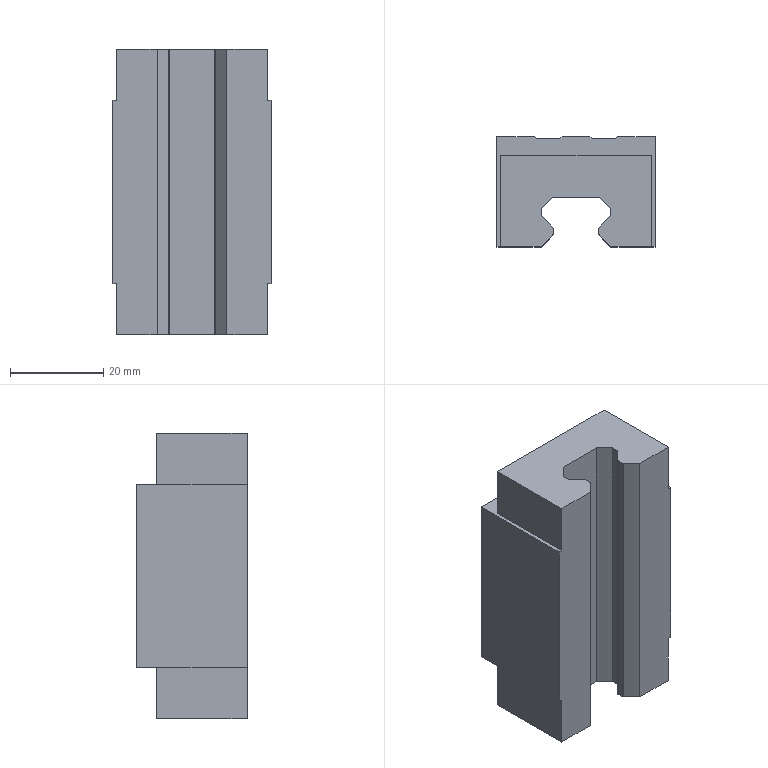Part | STEP file | Slider HGH15CA ( HGH15CA) | 1 solid | 50 faces | box 34 x 23.7 x 61.4 mm | volume 37112 mm3 | plane 38 | cylinder 12 | commonest cylinder face diameters 3.2 x8 0.8 x4
STEP:
#1=CARTESIAN_POINT('',(-26.228,-14.514,42.1));
#2=VERTEX_POINT('',#1);
#3=CARTESIAN_POINT('',(-26.228,-14.514,45.3));
#4=VERTEX_POINT('',#3);
#5=CARTESIAN_POINT('',(-26.228,-14.514,43.7));
#6=DIRECTION('',(0.,1.,0.));
#7=DIRECTION('',(0.,0.,1.));
#8=AXIS2_PLACEMENT_3D('',#5,#6,#7);
#9=CIRCLE('',#8,1.6);
#10=EDGE_CURVE('',#2,#4,#9,.T.);
#11=ORIENTED_EDGE('',*,*,#10,.F.);
#12=CARTESIAN_POINT('',(-26.228,-9.514,42.1));
#13=VERTEX_POINT('',#12);
#14=CARTESIAN_POINT('',(-26.228,-14.514,42.1));
#15=DIRECTION('',(0.,1.,0.));
#16=VECTOR('',#15,1000.);
#17=LINE('',#14,#16);
#18=EDGE_CURVE('',#2,#13,#17,.T.);
#19=ORIENTED_EDGE('',*,*,#18,.T.);
#20=CARTESIAN_POINT('',(-26.228,-9.514,45.3));
#21=VERTEX_POINT('',#20);
#22=CARTESIAN_POINT('',(-26.228,-9.514,43.7));
#23=DIRECTION('',(0.,1.,0.));
#24=DIRECTION('',(0.,0.,1.));
#25=AXIS2_PLACEMENT_3D('',#22,#23,#24);
#26=CIRCLE('',#25,1.6);
#27=EDGE_CURVE('',#13,#21,#26,.T.);
#28=ORIENTED_EDGE('',*,*,#27,.T.);
#29=CARTESIAN_POINT('',(-26.228,-14.514,45.3));
#30=DIRECTION('',(0.,1.,0.));
#31=VECTOR('',#30,1000.);
#32=LINE('',#29,#31);
#33=EDGE_CURVE('',#4,#21,#32,.T.);
#34=ORIENTED_EDGE('',*,*,#33,.F.);
#35=EDGE_LOOP('',(#11,#19,#28,#34));
#36=FACE_OUTER_BOUND('',#35,.T.);
#37=CARTESIAN_POINT('',(-26.228,-14.514,43.7));
#38=DIRECTION('',(0.,1.,0.));
#39=DIRECTION('',(0.,0.,1.));
#40=AXIS2_PLACEMENT_3D('',#37,#38,#39);
#41=CYLINDRICAL_SURFACE('',#40,1.6);
#42=ADVANCED_FACE('',(#36),#41,.F.);
#43=CARTESIAN_POINT('',(-26.228,-14.514,16.1));
#44=VERTEX_POINT('',#43);
#45=CARTESIAN_POINT('',(-26.228,-14.514,19.3));
#46=VERTEX_POINT('',#45);
#47=CARTESIAN_POINT('',(-26.228,-14.514,17.7));
#48=DIRECTION('',(0.,1.,0.));
#49=DIRECTION('',(0.,0.,1.));
#50=AXIS2_PLACEMENT_3D('',#47,#48,#49);
#51=CIRCLE('',#50,1.6);
#52=EDGE_CURVE('',#44,#46,#51,.T.);
#53=ORIENTED_EDGE('',*,*,#52,.F.);
#54=CARTESIAN_POINT('',(-26.228,-9.514,16.1));
#55=VERTEX_POINT('',#54);
#56=CARTESIAN_POINT('',(-26.228,-14.514,16.1));
#57=DIRECTION('',(0.,1.,0.));
#58=VECTOR('',#57,1000.);
#59=LINE('',#56,#58);
#60=EDGE_CURVE('',#44,#55,#59,.T.);
#61=ORIENTED_EDGE('',*,*,#60,.T.);
#62=CARTESIAN_POINT('',(-26.228,-9.514,19.3));
#63=VERTEX_POINT('',#62);
#64=CARTESIAN_POINT('',(-26.228,-9.514,17.7));
#65=DIRECTION('',(0.,1.,0.));
#66=DIRECTION('',(0.,0.,1.));
#67=AXIS2_PLACEMENT_3D('',#64,#65,#66);
#68=CIRCLE('',#67,1.6);
#69=EDGE_CURVE('',#55,#63,#68,.T.);
#70=ORIENTED_EDGE('',*,*,#69,.T.);
#71=CARTESIAN_POINT('',(-26.228,-14.514,19.3));
#72=DIRECTION('',(0.,1.,0.));
#73=VECTOR('',#72,1000.);
#74=LINE('',#71,#73);
#75=EDGE_CURVE('',#46,#63,#74,.T.);
#76=ORIENTED_EDGE('',*,*,#75,.F.);
#77=EDGE_LOOP('',(#53,#61,#70,#76));
#78=FACE_OUTER_BOUND('',#77,.T.);
#79=CARTESIAN_POINT('',(-26.228,-14.514,17.7));
#80=DIRECTION('',(0.,1.,0.));
#81=DIRECTION('',(0.,0.,1.));
#82=AXIS2_PLACEMENT_3D('',#79,#80,#81);
#83=CYLINDRICAL_SURFACE('',#82,1.6);
#84=ADVANCED_FACE('',(#78),#83,.F.);
#85=CARTESIAN_POINT('',(-0.2285,-14.514,42.1));
#86=VERTEX_POINT('',#85);
#87=CARTESIAN_POINT('',(-0.2285,-14.514,45.3));
#88=VERTEX_POINT('',#87);
#89=CARTESIAN_POINT('',(-0.2285,-14.514,43.7));
#90=DIRECTION('',(0.,1.,0.));
#91=DIRECTION('',(0.,0.,1.));
#92=AXIS2_PLACEMENT_3D('',#89,#90,#91);
#93=CIRCLE('',#92,1.6);
#94=EDGE_CURVE('',#86,#88,#93,.T.);
#95=ORIENTED_EDGE('',*,*,#94,.F.);
#96=CARTESIAN_POINT('',(-0.2285,-9.514,42.1));
#97=VERTEX_POINT('',#96);
#98=CARTESIAN_POINT('',(-0.2285,-14.514,42.1));
#99=DIRECTION('',(0.,1.,0.));
#100=VECTOR('',#99,1000.);
#101=LINE('',#98,#100);
#102=EDGE_CURVE('',#86,#97,#101,.T.);
#103=ORIENTED_EDGE('',*,*,#102,.T.);
#104=CARTESIAN_POINT('',(-0.2285,-9.514,45.3));
#105=VERTEX_POINT('',#104);
#106=CARTESIAN_POINT('',(-0.2285,-9.514,43.7));
#107=DIRECTION('',(0.,1.,0.));
#108=DIRECTION('',(0.,0.,1.));
#109=AXIS2_PLACEMENT_3D('',#106,#107,#108);
#110=CIRCLE('',#109,1.6);
#111=EDGE_CURVE('',#97,#105,#110,.T.);
#112=ORIENTED_EDGE('',*,*,#111,.T.);
#113=CARTESIAN_POINT('',(-0.2285,-14.514,45.3));
#114=DIRECTION('',(0.,1.,0.));
#115=VECTOR('',#114,1000.);
#116=LINE('',#113,#115);
#117=EDGE_CURVE('',#88,#105,#116,.T.);
#118=ORIENTED_EDGE('',*,*,#117,.F.);
#119=EDGE_LOOP('',(#95,#103,#112,#118));
#120=FACE_OUTER_BOUND('',#119,.T.);
#121=CARTESIAN_POINT('',(-0.2285,-14.514,43.7));
#122=DIRECTION('',(0.,1.,0.));
#123=DIRECTION('',(0.,0.,1.));
#124=AXIS2_PLACEMENT_3D('',#121,#122,#123);
#125=CYLINDRICAL_SURFACE('',#124,1.6);
#126=ADVANCED_FACE('',(#120),#125,.F.);
#127=CARTESIAN_POINT('',(-0.2285,-14.514,16.1));
#128=VERTEX_POINT('',#127);
#129=CARTESIAN_POINT('',(-0.2285,-14.514,19.3));
#130=VERTEX_POINT('',#129);
#131=CARTESIAN_POINT('',(-0.2285,-14.514,17.7));
#132=DIRECTION('',(0.,1.,0.));
#133=DIRECTION('',(0.,0.,1.));
#134=AXIS2_PLACEMENT_3D('',#131,#132,#133);
#135=CIRCLE('',#134,1.6);
#136=EDGE_CURVE('',#128,#130,#135,.T.);
#137=ORIENTED_EDGE('',*,*,#136,.F.);
#138=CARTESIAN_POINT('',(-0.2285,-9.514,16.1));
#139=VERTEX_POINT('',#138);
#140=CARTESIAN_POINT('',(-0.2285,-14.514,16.1));
#141=DIRECTION('',(0.,1.,0.));
#142=VECTOR('',#141,1000.);
#143=LINE('',#140,#142);
#144=EDGE_CURVE('',#128,#139,#143,.T.);
#145=ORIENTED_EDGE('',*,*,#144,.T.);
#146=CARTESIAN_POINT('',(-0.2285,-9.514,19.3));
#147=VERTEX_POINT('',#146);
#148=CARTESIAN_POINT('',(-0.2285,-9.514,17.7));
#149=DIRECTION('',(0.,1.,0.));
#150=DIRECTION('',(0.,0.,1.));
#151=AXIS2_PLACEMENT_3D('',#148,#149,#150);
#152=CIRCLE('',#151,1.6);
#153=EDGE_CURVE('',#139,#147,#152,.T.);
#154=ORIENTED_EDGE('',*,*,#153,.T.);
#155=CARTESIAN_POINT('',(-0.2285,-14.514,19.3));
#156=DIRECTION('',(0.,1.,0.));
#157=VECTOR('',#156,1000.);
#158=LINE('',#155,#157);
#159=EDGE_CURVE('',#130,#147,#158,.T.);
#160=ORIENTED_EDGE('',*,*,#159,.F.);
#161=EDGE_LOOP('',(#137,#145,#154,#160));
#162=FACE_OUTER_BOUND('',#161,.T.);
#163=CARTESIAN_POINT('',(-0.2285,-14.514,17.7));
#164=DIRECTION('',(0.,1.,0.));
#165=DIRECTION('',(0.,0.,1.));
#166=AXIS2_PLACEMENT_3D('',#163,#164,#165);
#167=CYLINDRICAL_SURFACE('',#166,1.6);
#168=ADVANCED_FACE('',(#162),#167,.F.);
#169=CARTESIAN_POINT('',(-29.428,-33.214,0.));
#170=VERTEX_POINT('',#169);
#171=CARTESIAN_POINT('',(-20.728,-33.214,0.));
#172=VERTEX_POINT('',#171);
#173=CARTESIAN_POINT('',(-29.428,-33.214,0.));
#174=DIRECTION('',(1.,0.,0.));
#175=VECTOR('',#174,1000.);
#176=LINE('',#173,#175);
#177=EDGE_CURVE('',#170,#172,#176,.T.);
#178=ORIENTED_EDGE('',*,*,#177,.T.);
#179=CARTESIAN_POINT('',(-20.728,-33.214,61.4));
#180=VERTEX_POINT('',#179);
#181=CARTESIAN_POINT('',(-20.728,-33.214,61.4));
#182=DIRECTION('',(0.,0.,-1.));
#183=VECTOR('',#182,1000.);
#184=LINE('',#181,#183);
#185=EDGE_CURVE('',#180,#172,#184,.T.);
#186=ORIENTED_EDGE('',*,*,#185,.F.);
#187=CARTESIAN_POINT('',(-29.428,-33.214,61.4));
#188=VERTEX_POINT('',#187);
#189=CARTESIAN_POINT('',(-29.428,-33.214,61.4));
#190=DIRECTION('',(1.,0.,0.));
#191=VECTOR('',#190,1000.);
#192=LINE('',#189,#191);
#193=EDGE_CURVE('',#188,#180,#192,.T.);
#194=ORIENTED_EDGE('',*,*,#193,.F.);
#195=CARTESIAN_POINT('',(-29.428,-33.214,50.4));
#196=VERTEX_POINT('',#195);
#197=CARTESIAN_POINT('',(-29.428,-33.214,50.4));
#198=DIRECTION('',(0.,0.,1.));
#199=VECTOR('',#198,1000.);
#200=LINE('',#197,#199);
#201=EDGE_CURVE('',#196,#188,#200,.T.);
#202=ORIENTED_EDGE('',*,*,#201,.F.);
#203=CARTESIAN_POINT('',(-30.228,-33.214,50.4));
#204=VERTEX_POINT('',#203);
#205=CARTESIAN_POINT('',(-30.228,-33.214,50.4));
#206=DIRECTION('',(1.,0.,0.));
#207=VECTOR('',#206,1000.);
#208=LINE('',#205,#207);
#209=EDGE_CURVE('',#204,#196,#208,.T.);
#210=ORIENTED_EDGE('',*,*,#209,.F.);
#211=CARTESIAN_POINT('',(-30.228,-33.214,11.));
#212=VERTEX_POINT('',#211);
#213=CARTESIAN_POINT('',(-30.228,-33.214,50.4));
#214=DIRECTION('',(0.,0.,-1.));
#215=VECTOR('',#214,1000.);
#216=LINE('',#213,#215);
#217=EDGE_CURVE('',#204,#212,#216,.T.);
#218=ORIENTED_EDGE('',*,*,#217,.T.);
#219=CARTESIAN_POINT('',(-29.428,-33.214,11.));
#220=VERTEX_POINT('',#219);
#221=CARTESIAN_POINT('',(-30.228,-33.214,11.));
#222=DIRECTION('',(1.,0.,0.));
#223=VECTOR('',#222,1000.);
#224=LINE('',#221,#223);
#225=EDGE_CURVE('',#212,#220,#224,.T.);
#226=ORIENTED_EDGE('',*,*,#225,.T.);
#227=CARTESIAN_POINT('',(-29.428,-33.214,11.));
#228=DIRECTION('',(0.,0.,-1.));
#229=VECTOR('',#228,1000.);
#230=LINE('',#227,#229);
#231=EDGE_CURVE('',#220,#170,#230,.T.);
#232=ORIENTED_EDGE('',*,*,#231,.T.);
#233=EDGE_LOOP('',(#178,#186,#194,#202,#210,#218,#226,#232));
#234=FACE_OUTER_BOUND('',#233,.T.);
#235=CARTESIAN_POINT('',(-29.428,-33.214,11.));
#236=DIRECTION('',(0.,1.,0.));
#237=DIRECTION('',(0.,0.,1.));
#238=AXIS2_PLACEMENT_3D('',#235,#236,#237);
#239=PLANE('',#238);
#240=ADVANCED_FACE('',(#234),#239,.F.);
#241=CARTESIAN_POINT('',(-21.728,-10.014,11.));
#242=VERTEX_POINT('',#241);
#243=CARTESIAN_POINT('',(-22.228,-9.514,11.));
#244=VERTEX_POINT('',#243);
#245=CARTESIAN_POINT('',(-14.378,-17.364,11.));
#246=DIRECTION('',(-0.7071,0.7071,0.));
#247=VECTOR('',#246,1000.);
#248=LINE('',#245,#247);
#249=EDGE_CURVE('',#242,#244,#248,.T.);
#250=ORIENTED_EDGE('',*,*,#249,.F.);
#251=CARTESIAN_POINT('',(-16.728,-10.014,11.));
#252=VERTEX_POINT('',#251);
#253=CARTESIAN_POINT('',(-30.228,-10.014,11.));
#254=DIRECTION('',(-1.,0.,0.));
#255=VECTOR('',#254,1000.);
#256=LINE('',#253,#255);
#257=EDGE_CURVE('',#252,#242,#256,.T.);
#258=ORIENTED_EDGE('',*,*,#257,.F.);
#259=CARTESIAN_POINT('',(-16.228,-9.514,11.));
#260=VERTEX_POINT('',#259);
#261=CARTESIAN_POINT('',(-35.078,-28.364,11.));
#262=DIRECTION('',(-0.7071,-0.7071,0.));
#263=VECTOR('',#262,1000.);
#264=LINE('',#261,#263);
#265=EDGE_CURVE('',#260,#252,#264,.T.);
#266=ORIENTED_EDGE('',*,*,#265,.F.);
#267=CARTESIAN_POINT('',(-10.228,-9.514,11.));
#268=VERTEX_POINT('',#267);
#269=CARTESIAN_POINT('',(-30.228,-9.514,11.));
#270=DIRECTION('',(-1.,0.,0.));
#271=VECTOR('',#270,1000.);
#272=LINE('',#269,#271);
#273=EDGE_CURVE('',#268,#260,#272,.T.);
#274=ORIENTED_EDGE('',*,*,#273,.F.);
#275=CARTESIAN_POINT('',(-9.728,-10.014,11.));
#276=VERTEX_POINT('',#275);
#277=CARTESIAN_POINT('',(-8.378,-11.364,11.));
#278=DIRECTION('',(0.7071,-0.7071,0.));
#279=VECTOR('',#278,1000.);
#280=LINE('',#277,#279);
#281=EDGE_CURVE('',#268,#276,#280,.T.);
#282=ORIENTED_EDGE('',*,*,#281,.T.);
#283=CARTESIAN_POINT('',(-4.728,-10.014,11.));
#284=VERTEX_POINT('',#283);
#285=CARTESIAN_POINT('',(-30.228,-10.014,11.));
#286=DIRECTION('',(1.,0.,0.));
#287=VECTOR('',#286,1000.);
#288=LINE('',#285,#287);
#289=EDGE_CURVE('',#276,#284,#288,.T.);
#290=ORIENTED_EDGE('',*,*,#289,.T.);
#291=CARTESIAN_POINT('',(-4.228,-9.514,11.));
#292=VERTEX_POINT('',#291);
#293=CARTESIAN_POINT('',(-29.078,-34.364,11.));
#294=DIRECTION('',(0.7071,0.7071,0.));
#295=VECTOR('',#294,1000.);
#296=LINE('',#293,#295);
#297=EDGE_CURVE('',#284,#292,#296,.T.);
#298=ORIENTED_EDGE('',*,*,#297,.T.);
#299=CARTESIAN_POINT('',(3.772,-9.514,11.));
#300=VERTEX_POINT('',#299);
#301=CARTESIAN_POINT('',(-30.228,-9.514,11.));
#302=DIRECTION('',(-1.,0.,0.));
#303=VECTOR('',#302,1000.);
#304=LINE('',#301,#303);
#305=EDGE_CURVE('',#300,#292,#304,.T.);
#306=ORIENTED_EDGE('',*,*,#305,.F.);
#307=CARTESIAN_POINT('',(3.772,-33.214,11.));
#308=VERTEX_POINT('',#307);
#309=CARTESIAN_POINT('',(3.772,-9.514,11.));
#310=DIRECTION('',(0.,1.,0.));
#311=VECTOR('',#310,1000.);
#312=LINE('',#309,#311);
#313=EDGE_CURVE('',#308,#300,#312,.T.);
#314=ORIENTED_EDGE('',*,*,#313,.F.);
#315=CARTESIAN_POINT('',(2.972,-33.214,11.));
#316=VERTEX_POINT('',#315);
#317=CARTESIAN_POINT('',(-30.228,-33.214,11.));
#318=DIRECTION('',(1.,0.,0.));
#319=VECTOR('',#318,1000.);
#320=LINE('',#317,#319);
#321=EDGE_CURVE('',#316,#308,#320,.T.);
#322=ORIENTED_EDGE('',*,*,#321,.F.);
#323=CARTESIAN_POINT('',(2.972,-13.684,11.));
#324=VERTEX_POINT('',#323);
#325=CARTESIAN_POINT('',(2.972,-13.684,11.));
#326=DIRECTION('',(0.,1.,0.));
#327=VECTOR('',#326,1000.);
#328=LINE('',#325,#327);
#329=EDGE_CURVE('',#316,#324,#328,.T.);
#330=ORIENTED_EDGE('',*,*,#329,.T.);
#331=CARTESIAN_POINT('',(-29.428,-13.684,11.));
#332=VERTEX_POINT('',#331);
#333=CARTESIAN_POINT('',(-29.428,-13.684,11.));
#334=DIRECTION('',(-1.,0.,0.));
#335=VECTOR('',#334,1000.);
#336=LINE('',#333,#335);
#337=EDGE_CURVE('',#324,#332,#336,.T.);
#338=ORIENTED_EDGE('',*,*,#337,.T.);
#339=CARTESIAN_POINT('',(-29.428,-13.684,11.));
#340=DIRECTION('',(0.,-1.,0.));
#341=VECTOR('',#340,1000.);
#342=LINE('',#339,#341);
#343=EDGE_CURVE('',#332,#220,#342,.T.);
#344=ORIENTED_EDGE('',*,*,#343,.T.);
#345=ORIENTED_EDGE('',*,*,#225,.F.);
#346=CARTESIAN_POINT('',(-30.228,-9.514,11.));
#347=VERTEX_POINT('',#346);
#348=CARTESIAN_POINT('',(-30.228,-9.514,11.));
#349=DIRECTION('',(0.,-1.,0.));
#350=VECTOR('',#349,1000.);
#351=LINE('',#348,#350);
#352=EDGE_CURVE('',#347,#212,#351,.T.);
#353=ORIENTED_EDGE('',*,*,#352,.F.);
#354=CARTESIAN_POINT('',(-30.228,-9.514,11.));
#355=DIRECTION('',(-1.,0.,0.));
#356=VECTOR('',#355,1000.);
#357=LINE('',#354,#356);
#358=EDGE_CURVE('',#244,#347,#357,.T.);
#359=ORIENTED_EDGE('',*,*,#358,.F.);
#360=EDGE_LOOP('',(#250,#258,#266,#274,#282,#290,#298,#306,#314,#322,#330,#338,#344,#345,#353,#359));
#361=FACE_OUTER_BOUND('',#360,.T.);
#362=CARTESIAN_POINT('',(-30.228,-33.214,11.));
#363=DIRECTION('',(0.,0.,1.));
#364=DIRECTION('',(1.,0.,0.));
#365=AXIS2_PLACEMENT_3D('',#362,#363,#364);
#366=PLANE('',#365);
#367=ADVANCED_FACE('',(#361),#366,.F.);
#368=CARTESIAN_POINT('',(-26.228,-9.514,43.7));
#369=DIRECTION('',(0.,1.,0.));
#370=DIRECTION('',(0.,0.,1.));
#371=AXIS2_PLACEMENT_3D('',#368,#369,#370);
#372=CIRCLE('',#371,1.6);
#373=EDGE_CURVE('',#21,#13,#372,.T.);
#374=ORIENTED_EDGE('',*,*,#373,.F.);
#375=ORIENTED_EDGE('',*,*,#27,.F.);
#376=EDGE_LOOP('',(#374,#375));
#377=FACE_BOUND('',#376,.T.);
#378=CARTESIAN_POINT('',(-26.228,-9.514,17.7));
#379=DIRECTION('',(0.,1.,0.));
#380=DIRECTION('',(0.,0.,1.));
#381=AXIS2_PLACEMENT_3D('',#378,#379,#380);
#382=CIRCLE('',#381,1.6);
#383=EDGE_CURVE('',#63,#55,#382,.T.);
#384=ORIENTED_EDGE('',*,*,#383,.F.);
#385=ORIENTED_EDGE('',*,*,#69,.F.);
#386=EDGE_LOOP('',(#384,#385));
#387=FACE_BOUND('',#386,.T.);
#388=CARTESIAN_POINT('',(-22.228,-9.514,50.4));
#389=VERTEX_POINT('',#388);
#390=CARTESIAN_POINT('',(-22.228,-9.514,-0.000025));
#391=DIRECTION('',(0.,0.,1.));
#392=VECTOR('',#391,1000.);
#393=LINE('',#390,#392);
#394=EDGE_CURVE('',#244,#389,#393,.T.);
#395=ORIENTED_EDGE('',*,*,#394,.F.);
#396=ORIENTED_EDGE('',*,*,#358,.T.);
#397=CARTESIAN_POINT('',(-30.228,-9.514,50.4));
#398=VERTEX_POINT('',#397);
#399=CARTESIAN_POINT('',(-30.228,-9.514,50.4));
#400=DIRECTION('',(0.,0.,-1.));
#401=VECTOR('',#400,1000.);
#402=LINE('',#399,#401);
#403=EDGE_CURVE('',#398,#347,#402,.T.);
#404=ORIENTED_EDGE('',*,*,#403,.F.);
#405=CARTESIAN_POINT('',(-30.228,-9.514,50.4));
#406=DIRECTION('',(-1.,0.,0.));
#407=VECTOR('',#406,1000.);
#408=LINE('',#405,#407);
#409=EDGE_CURVE('',#389,#398,#408,.T.);
#410=ORIENTED_EDGE('',*,*,#409,.F.);
#411=EDGE_LOOP('',(#395,#396,#404,#410));
#412=FACE_OUTER_BOUND('',#411,.T.);
#413=CARTESIAN_POINT('',(-30.228,-9.514,50.4));
#414=DIRECTION('',(0.,-1.,0.));
#415=DIRECTION('',(0.,0.,-1.));
#416=AXIS2_PLACEMENT_3D('',#413,#414,#415);
#417=PLANE('',#416);
#418=ADVANCED_FACE('',(#377,#387,#412),#417,.F.);
#419=CARTESIAN_POINT('',(-16.228,-9.514,50.4));
#420=VERTEX_POINT('',#419);
#421=CARTESIAN_POINT('',(-16.228,-9.514,-0.000025));
#422=DIRECTION('',(0.,0.,1.));
#423=VECTOR('',#422,1000.);
#424=LINE('',#421,#423);
#425=EDGE_CURVE('',#260,#420,#424,.T.);
#426=ORIENTED_EDGE('',*,*,#425,.T.);
#427=CARTESIAN_POINT('',(-10.228,-9.514,50.4));
#428=VERTEX_POINT('',#427);
#429=CARTESIAN_POINT('',(-30.228,-9.514,50.4));
#430=DIRECTION('',(-1.,0.,0.));
#431=VECTOR('',#430,1000.);
#432=LINE('',#429,#431);
#433=EDGE_CURVE('',#428,#420,#432,.T.);
#434=ORIENTED_EDGE('',*,*,#433,.F.);
#435=CARTESIAN_POINT('',(-10.228,-9.514,-0.000025));
#436=DIRECTION('',(0.,0.,1.));
#437=VECTOR('',#436,1000.);
#438=LINE('',#435,#437);
#439=EDGE_CURVE('',#268,#428,#438,.T.);
#440=ORIENTED_EDGE('',*,*,#439,.F.);
#441=ORIENTED_EDGE('',*,*,#273,.T.);
#442=EDGE_LOOP('',(#426,#434,#440,#441));
#443=FACE_OUTER_BOUND('',#442,.T.);
#444=CARTESIAN_POINT('',(-30.228,-9.514,50.4));
#445=DIRECTION('',(0.,-1.,0.));
#446=DIRECTION('',(0.,0.,-1.));
#447=AXIS2_PLACEMENT_3D('',#444,#445,#446);
#448=PLANE('',#447);
#449=ADVANCED_FACE('',(#443),#448,.F.);
#450=CARTESIAN_POINT('',(-16.728,-10.014,50.4));
#451=VERTEX_POINT('',#450);
#452=CARTESIAN_POINT('',(-21.728,-10.014,50.4));
#453=VERTEX_POINT('',#452);
#454=CARTESIAN_POINT('',(-16.728,-10.014,50.4));
#455=DIRECTION('',(-1.,0.,0.));
#456=VECTOR('',#455,1000.);
#457=LINE('',#454,#456);
#458=EDGE_CURVE('',#451,#453,#457,.T.);
#459=ORIENTED_EDGE('',*,*,#458,.T.);
#460=CARTESIAN_POINT('',(-21.728,-10.014,50.4));
#461=DIRECTION('',(-0.7071,0.7071,0.));
#462=VECTOR('',#461,1000.);
#463=LINE('',#460,#462);
#464=EDGE_CURVE('',#453,#389,#463,.T.);
#465=ORIENTED_EDGE('',*,*,#464,.T.);
#466=ORIENTED_EDGE('',*,*,#409,.T.);
#467=CARTESIAN_POINT('',(-30.228,-9.514,50.4));
#468=DIRECTION('',(0.,-1.,0.));
#469=VECTOR('',#468,1000.);
#470=LINE('',#467,#469);
#471=EDGE_CURVE('',#398,#204,#470,.T.);
#472=ORIENTED_EDGE('',*,*,#471,.T.);
#473=ORIENTED_EDGE('',*,*,#209,.T.);
#474=CARTESIAN_POINT('',(-29.428,-13.684,50.4));
#475=VERTEX_POINT('',#474);
#476=CARTESIAN_POINT('',(-29.428,-13.684,50.4));
#477=DIRECTION('',(0.,-1.,0.));
#478=VECTOR('',#477,1000.);
#479=LINE('',#476,#478);
#480=EDGE_CURVE('',#475,#196,#479,.T.);
#481=ORIENTED_EDGE('',*,*,#480,.F.);
#482=CARTESIAN_POINT('',(2.972,-13.684,50.4));
#483=VERTEX_POINT('',#482);
#484=CARTESIAN_POINT('',(-29.428,-13.684,50.4));
#485=DIRECTION('',(-1.,0.,0.));
#486=VECTOR('',#485,1000.);
#487=LINE('',#484,#486);
#488=EDGE_CURVE('',#483,#475,#487,.T.);
#489=ORIENTED_EDGE('',*,*,#488,.F.);
#490=CARTESIAN_POINT('',(2.972,-33.214,50.4));
#491=VERTEX_POINT('',#490);
#492=CARTESIAN_POINT('',(2.972,-13.684,50.4));
#493=DIRECTION('',(0.,1.,0.));
#494=VECTOR('',#493,1000.);
#495=LINE('',#492,#494);
#496=EDGE_CURVE('',#491,#483,#495,.T.);
#497=ORIENTED_EDGE('',*,*,#496,.F.);
#498=CARTESIAN_POINT('',(3.772,-33.214,50.4));
#499=VERTEX_POINT('',#498);
#500=CARTESIAN_POINT('',(-30.228,-33.214,50.4));
#501=DIRECTION('',(1.,0.,0.));
#502=VECTOR('',#501,1000.);
#503=LINE('',#500,#502);
#504=EDGE_CURVE('',#491,#499,#503,.T.);
#505=ORIENTED_EDGE('',*,*,#504,.T.);
#506=CARTESIAN_POINT('',(3.772,-9.514,50.4));
#507=VERTEX_POINT('',#506);
#508=CARTESIAN_POINT('',(3.772,-9.514,50.4));
#509=DIRECTION('',(0.,1.,0.));
#510=VECTOR('',#509,1000.);
#511=LINE('',#508,#510);
#512=EDGE_CURVE('',#499,#507,#511,.T.);
#513=ORIENTED_EDGE('',*,*,#512,.T.);
#514=CARTESIAN_POINT('',(-4.228,-9.514,50.4));
#515=VERTEX_POINT('',#514);
#516=CARTESIAN_POINT('',(-30.228,-9.514,50.4));
#517=DIRECTION('',(-1.,0.,0.));
#518=VECTOR('',#517,1000.);
#519=LINE('',#516,#518);
#520=EDGE_CURVE('',#507,#515,#519,.T.);
#521=ORIENTED_EDGE('',*,*,#520,.T.);
#522=CARTESIAN_POINT('',(-4.728,-10.014,50.4));
#523=VERTEX_POINT('',#522);
#524=CARTESIAN_POINT('',(-4.728,-10.014,50.4));
#525=DIRECTION('',(0.7071,0.7071,0.));
#526=VECTOR('',#525,1000.);
#527=LINE('',#524,#526);
#528=EDGE_CURVE('',#523,#515,#527,.T.);
#529=ORIENTED_EDGE('',*,*,#528,.F.);
#530=CARTESIAN_POINT('',(-9.728,-10.014,50.4));
#531=VERTEX_POINT('',#530);
#532=CARTESIAN_POINT('',(-9.728,-10.014,50.4));
#533=DIRECTION('',(1.,0.,0.));
#534=VECTOR('',#533,1000.);
#535=LINE('',#532,#534);
#536=EDGE_CURVE('',#531,#523,#535,.T.);
#537=ORIENTED_EDGE('',*,*,#536,.F.);
#538=CARTESIAN_POINT('',(-9.728,-10.014,50.4));
#539=DIRECTION('',(0.7071,-0.7071,0.));
#540=VECTOR('',#539,1000.);
#541=LINE('',#538,#540);
#542=EDGE_CURVE('',#428,#531,#541,.T.);
#543=ORIENTED_EDGE('',*,*,#542,.F.);
#544=ORIENTED_EDGE('',*,*,#433,.T.);
#545=CARTESIAN_POINT('',(-16.728,-10.014,50.4));
#546=DIRECTION('',(-0.7071,-0.7071,0.));
#547=VECTOR('',#546,1000.);
#548=LINE('',#545,#547);
#549=EDGE_CURVE('',#420,#451,#548,.T.);
#550=ORIENTED_EDGE('',*,*,#549,.T.);
#551=EDGE_LOOP('',(#459,#465,#466,#472,#473,#481,#489,#497,#505,#513,#521,#529,#537,#543,#544,#550));
#552=FACE_OUTER_BOUND('',#551,.T.);
#553=CARTESIAN_POINT('',(-30.228,-33.214,50.4));
#554=DIRECTION('',(0.,0.,1.));
#555=DIRECTION('',(1.,0.,0.));
#556=AXIS2_PLACEMENT_3D('',#553,#554,#555);
#557=PLANE('',#556);
#558=ADVANCED_FACE('',(#552),#557,.T.);
#559=CARTESIAN_POINT('',(-0.2285,-9.514,43.7));
#560=DIRECTION('',(0.,1.,0.));
#561=DIRECTION('',(0.,0.,1.));
#562=AXIS2_PLACEMENT_3D('',#559,#560,#561);
#563=CIRCLE('',#562,1.6);
#564=EDGE_CURVE('',#105,#97,#563,.T.);
#565=ORIENTED_EDGE('',*,*,#564,.F.);
#566=ORIENTED_EDGE('',*,*,#111,.F.);
#567=EDGE_LOOP('',(#565,#566));
#568=FACE_BOUND('',#567,.T.);
#569=CARTESIAN_POINT('',(-0.2285,-9.514,17.7));
#570=DIRECTION('',(0.,1.,0.));
#571=DIRECTION('',(0.,0.,1.));
#572=AXIS2_PLACEMENT_3D('',#569,#570,#571);
#573=CIRCLE('',#572,1.6);
#574=EDGE_CURVE('',#147,#139,#573,.T.);
#575=ORIENTED_EDGE('',*,*,#574,.F.);
#576=ORIENTED_EDGE('',*,*,#153,.F.);
#577=EDGE_LOOP('',(#575,#576));
#578=FACE_BOUND('',#577,.T.);
#579=ORIENTED_EDGE('',*,*,#305,.T.);
#580=CARTESIAN_POINT('',(-4.228,-9.514,-0.000025));
#581=DIRECTION('',(0.,0.,1.));
#582=VECTOR('',#581,1000.);
#583=LINE('',#580,#582);
#584=EDGE_CURVE('',#292,#515,#583,.T.);
#585=ORIENTED_EDGE('',*,*,#584,.T.);
#586=ORIENTED_EDGE('',*,*,#520,.F.);
#587=CARTESIAN_POINT('',(3.772,-9.514,50.4));
#588=DIRECTION('',(0.,0.,-1.));
#589=VECTOR('',#588,1000.);
#590=LINE('',#587,#589);
#591=EDGE_CURVE('',#507,#300,#590,.T.);
#592=ORIENTED_EDGE('',*,*,#591,.T.);
#593=EDGE_LOOP('',(#579,#585,#586,#592));
#594=FACE_OUTER_BOUND('',#593,.T.);
#595=CARTESIAN_POINT('',(-30.228,-9.514,50.4));
#596=DIRECTION('',(0.,-1.,0.));
#597=DIRECTION('',(0.,0.,-1.));
#598=AXIS2_PLACEMENT_3D('',#595,#596,#597);
#599=PLANE('',#598);
#600=ADVANCED_FACE('',(#568,#578,#594),#599,.F.);
#601=CARTESIAN_POINT('',(-29.428,-13.684,0.));
#602=VERTEX_POINT('',#601);
#603=CARTESIAN_POINT('',(-29.428,-13.684,0.));
#604=DIRECTION('',(0.,-1.,0.));
#605=VECTOR('',#604,1000.);
#606=LINE('',#603,#605);
#607=EDGE_CURVE('',#602,#170,#606,.T.);
#608=ORIENTED_EDGE('',*,*,#607,.T.);
#609=ORIENTED_EDGE('',*,*,#231,.F.);
#610=ORIENTED_EDGE('',*,*,#343,.F.);
#611=CARTESIAN_POINT('',(-29.428,-13.684,11.));
#612=DIRECTION('',(0.,0.,-1.));
#613=VECTOR('',#612,1000.);
#614=LINE('',#611,#613);
#615=EDGE_CURVE('',#332,#602,#614,.T.);
#616=ORIENTED_EDGE('',*,*,#615,.T.);
#617=EDGE_LOOP('',(#608,#609,#610,#616));
#618=FACE_OUTER_BOUND('',#617,.T.);
#619=CARTESIAN_POINT('',(-29.428,-13.684,11.));
#620=DIRECTION('',(1.,0.,0.));
#621=DIRECTION('',(0.,1.,0.));
#622=AXIS2_PLACEMENT_3D('',#619,#620,#621);
#623=PLANE('',#622);
#624=ADVANCED_FACE('',(#618),#623,.F.);
#625=CARTESIAN_POINT('',(-5.728,-33.214,61.4));
#626=VERTEX_POINT('',#625);
#627=CARTESIAN_POINT('',(2.972,-33.214,61.4));
#628=VERTEX_POINT('',#627);
#629=CARTESIAN_POINT('',(-29.428,-33.214,61.4));
#630=DIRECTION('',(1.,0.,0.));
#631=VECTOR('',#630,1000.);
#632=LINE('',#629,#631);
#633=EDGE_CURVE('',#626,#628,#632,.T.);
#634=ORIENTED_EDGE('',*,*,#633,.F.);
#635=CARTESIAN_POINT('',(-5.728,-33.214,0.));
#636=VERTEX_POINT('',#635);
#637=CARTESIAN_POINT('',(-5.728,-33.214,61.4));
#638=DIRECTION('',(0.,0.,-1.));
#639=VECTOR('',#638,1000.);
#640=LINE('',#637,#639);
#641=EDGE_CURVE('',#626,#636,#640,.T.);
#642=ORIENTED_EDGE('',*,*,#641,.T.);
#643=CARTESIAN_POINT('',(2.972,-33.214,0.));
#644=VERTEX_POINT('',#643);
#645=CARTESIAN_POINT('',(-29.428,-33.214,0.));
#646=DIRECTION('',(1.,0.,0.));
#647=VECTOR('',#646,1000.);
#648=LINE('',#645,#647);
#649=EDGE_CURVE('',#636,#644,#648,.T.);
#650=ORIENTED_EDGE('',*,*,#649,.T.);
#651=CARTESIAN_POINT('',(2.972,-33.214,11.));
#652=DIRECTION('',(0.,0.,-1.));
#653=VECTOR('',#652,1000.);
#654=LINE('',#651,#653);
#655=EDGE_CURVE('',#316,#644,#654,.T.);
#656=ORIENTED_EDGE('',*,*,#655,.F.);
#657=ORIENTED_EDGE('',*,*,#321,.T.);
#658=CARTESIAN_POINT('',(3.772,-33.214,50.4));
#659=DIRECTION('',(0.,0.,-1.));
#660=VECTOR('',#659,1000.);
#661=LINE('',#658,#660);
#662=EDGE_CURVE('',#499,#308,#661,.T.);
#663=ORIENTED_EDGE('',*,*,#662,.F.);
#664=ORIENTED_EDGE('',*,*,#504,.F.);
#665=CARTESIAN_POINT('',(2.972,-33.214,50.4));
#666=DIRECTION('',(0.,0.,1.));
#667=VECTOR('',#666,1000.);
#668=LINE('',#665,#667);
#669=EDGE_CURVE('',#491,#628,#668,.T.);
#670=ORIENTED_EDGE('',*,*,#669,.T.);
#671=EDGE_LOOP('',(#634,#642,#650,#656,#657,#663,#664,#670));
#672=FACE_OUTER_BOUND('',#671,.T.);
#673=CARTESIAN_POINT('',(-29.428,-33.214,11.));
#674=DIRECTION('',(0.,1.,0.));
#675=DIRECTION('',(0.,0.,1.));
#676=AXIS2_PLACEMENT_3D('',#673,#674,#675);
#677=PLANE('',#676);
#678=ADVANCED_FACE('',(#672),#677,.F.);
#679=CARTESIAN_POINT('',(2.972,-13.684,0.));
#680=VERTEX_POINT('',#679);
#681=CARTESIAN_POINT('',(2.972,-13.684,0.));
#682=DIRECTION('',(0.,1.,0.));
#683=VECTOR('',#682,1000.);
#684=LINE('',#681,#683);
#685=EDGE_CURVE('',#644,#680,#684,.T.);
#686=ORIENTED_EDGE('',*,*,#685,.T.);
#687=CARTESIAN_POINT('',(2.972,-13.684,11.));
#688=DIRECTION('',(0.,0.,-1.));
#689=VECTOR('',#688,1000.);
#690=LINE('',#687,#689);
#691=EDGE_CURVE('',#324,#680,#690,.T.);
#692=ORIENTED_EDGE('',*,*,#691,.F.);
#693=ORIENTED_EDGE('',*,*,#329,.F.);
#694=ORIENTED_EDGE('',*,*,#655,.T.);
#695=EDGE_LOOP('',(#686,#692,#693,#694));
#696=FACE_OUTER_BOUND('',#695,.T.);
#697=CARTESIAN_POINT('',(2.972,-13.684,11.));
#698=DIRECTION('',(-1.,0.,0.));
#699=DIRECTION('',(0.,0.,1.));
#700=AXIS2_PLACEMENT_3D('',#697,#698,#699);
#701=PLANE('',#700);
#702=ADVANCED_FACE('',(#696),#701,.F.);
#703=CARTESIAN_POINT('',(-29.428,-13.684,0.));
#704=DIRECTION('',(-1.,0.,0.));
#705=VECTOR('',#704,1000.);
#706=LINE('',#703,#705);
#707=EDGE_CURVE('',#680,#602,#706,.T.);
#708=ORIENTED_EDGE('',*,*,#707,.T.);
#709=ORIENTED_EDGE('',*,*,#615,.F.);
#710=ORIENTED_EDGE('',*,*,#337,.F.);
#711=ORIENTED_EDGE('',*,*,#691,.T.);
#712=EDGE_LOOP('',(#708,#709,#710,#711));
#713=FACE_OUTER_BOUND('',#712,.T.);
#714=CARTESIAN_POINT('',(-29.428,-13.684,11.));
#715=DIRECTION('',(0.,-1.,0.));
#716=DIRECTION('',(0.,0.,-1.));
#717=AXIS2_PLACEMENT_3D('',#714,#715,#716);
#718=PLANE('',#717);
#719=ADVANCED_FACE('',(#713),#718,.F.);
#720=CARTESIAN_POINT('',(-18.153,-30.473,0.));
#721=VERTEX_POINT('',#720);
#722=CARTESIAN_POINT('',(-18.153,-29.245,0.));
#723=VERTEX_POINT('',#722);
#724=CARTESIAN_POINT('',(-18.153,-30.639,0.));
#725=DIRECTION('',(0.,1.,0.));
#726=VECTOR('',#725,1000.);
#727=LINE('',#724,#726);
#728=EDGE_CURVE('',#721,#723,#727,.T.);
#729=ORIENTED_EDGE('',*,*,#728,.F.);
#730=CARTESIAN_POINT('',(-18.271,-30.756,0.));
#731=VERTEX_POINT('',#730);
#732=CARTESIAN_POINT('',(-18.553,-30.473,0.));
#733=DIRECTION('',(0.,0.,-1.));
#734=DIRECTION('',(1.,0.,0.));
#735=AXIS2_PLACEMENT_3D('',#732,#733,#734);
#736=CIRCLE('',#735,0.4);
#737=EDGE_CURVE('',#721,#731,#736,.T.);
#738=ORIENTED_EDGE('',*,*,#737,.T.);
#739=CARTESIAN_POINT('',(-20.728,-33.214,0.));
#740=DIRECTION('',(0.7071,0.7071,0.));
#741=VECTOR('',#740,1000.);
#742=LINE('',#739,#741);
#743=EDGE_CURVE('',#172,#731,#742,.T.);
#744=ORIENTED_EDGE('',*,*,#743,.F.);
#745=ORIENTED_EDGE('',*,*,#177,.F.);
#746=ORIENTED_EDGE('',*,*,#607,.F.);
#747=ORIENTED_EDGE('',*,*,#707,.F.);
#748=ORIENTED_EDGE('',*,*,#685,.F.);
#749=ORIENTED_EDGE('',*,*,#649,.F.);
#750=CARTESIAN_POINT('',(-8.186,-30.756,0.));
#751=VERTEX_POINT('',#750);
#752=CARTESIAN_POINT('',(-5.728,-33.214,0.));
#753=DIRECTION('',(0.7071,-0.7071,0.));
#754=VECTOR('',#753,1000.);
#755=LINE('',#752,#754);
#756=EDGE_CURVE('',#751,#636,#755,.T.);
#757=ORIENTED_EDGE('',*,*,#756,.F.);
#758=CARTESIAN_POINT('',(-8.303,-30.473,0.));
#759=VERTEX_POINT('',#758);
#760=CARTESIAN_POINT('',(-7.903,-30.473,0.));
#761=DIRECTION('',(0.,0.,-1.));
#762=DIRECTION('',(1.,0.,0.));
#763=AXIS2_PLACEMENT_3D('',#760,#761,#762);
#764=CIRCLE('',#763,0.4);
#765=EDGE_CURVE('',#751,#759,#764,.T.);
#766=ORIENTED_EDGE('',*,*,#765,.T.);
#767=CARTESIAN_POINT('',(-8.303,-29.245,0.));
#768=VERTEX_POINT('',#767);
#769=CARTESIAN_POINT('',(-8.303,-30.639,0.));
#770=DIRECTION('',(0.,-1.,0.));
#771=VECTOR('',#770,1000.);
#772=LINE('',#769,#771);
#773=EDGE_CURVE('',#768,#759,#772,.T.);
#774=ORIENTED_EDGE('',*,*,#773,.F.);
#775=CARTESIAN_POINT('',(-8.186,-28.962,0.));
#776=VERTEX_POINT('',#775);
#777=CARTESIAN_POINT('',(-7.903,-29.245,0.));
#778=DIRECTION('',(0.,0.,-1.));
#779=DIRECTION('',(1.,0.,0.));
#780=AXIS2_PLACEMENT_3D('',#777,#778,#779);
#781=CIRCLE('',#780,0.4);
#782=EDGE_CURVE('',#768,#776,#781,.T.);
#783=ORIENTED_EDGE('',*,*,#782,.T.);
#784=CARTESIAN_POINT('',(-5.728,-26.504,0.));
#785=VERTEX_POINT('',#784);
#786=CARTESIAN_POINT('',(-8.303,-29.079,0.));
#787=DIRECTION('',(-0.7071,-0.7071,0.));
#788=VECTOR('',#787,1000.);
#789=LINE('',#786,#788);
#790=EDGE_CURVE('',#785,#776,#789,.T.);
#791=ORIENTED_EDGE('',*,*,#790,.F.);
#792=CARTESIAN_POINT('',(-5.728,-24.964,0.));
#793=VERTEX_POINT('',#792);
#794=CARTESIAN_POINT('',(-5.728,-26.504,0.));
#795=DIRECTION('',(0.,-1.,0.));
#796=VECTOR('',#795,1000.);
#797=LINE('',#794,#796);
#798=EDGE_CURVE('',#793,#785,#797,.T.);
#799=ORIENTED_EDGE('',*,*,#798,.F.);
#800=CARTESIAN_POINT('',(-8.178,-22.514,0.));
#801=VERTEX_POINT('',#800);
#802=CARTESIAN_POINT('',(-5.728,-24.964,0.));
#803=DIRECTION('',(0.7071,-0.7071,0.));
#804=VECTOR('',#803,1000.);
#805=LINE('',#802,#804);
#806=EDGE_CURVE('',#801,#793,#805,.T.);
#807=ORIENTED_EDGE('',*,*,#806,.F.);
#808=CARTESIAN_POINT('',(-18.278,-22.514,0.));
#809=VERTEX_POINT('',#808);
#810=CARTESIAN_POINT('',(-18.278,-22.514,0.));
#811=DIRECTION('',(1.,0.,0.));
#812=VECTOR('',#811,1000.);
#813=LINE('',#810,#812);
#814=EDGE_CURVE('',#809,#801,#813,.T.);
#815=ORIENTED_EDGE('',*,*,#814,.F.);
#816=CARTESIAN_POINT('',(-20.728,-24.964,0.));
#817=VERTEX_POINT('',#816);
#818=CARTESIAN_POINT('',(-20.728,-24.964,0.));
#819=DIRECTION('',(0.7071,0.7071,0.));
#820=VECTOR('',#819,1000.);
#821=LINE('',#818,#820);
#822=EDGE_CURVE('',#817,#809,#821,.T.);
#823=ORIENTED_EDGE('',*,*,#822,.F.);
#824=CARTESIAN_POINT('',(-20.728,-26.504,0.));
#825=VERTEX_POINT('',#824);
#826=CARTESIAN_POINT('',(-20.728,-26.504,0.));
#827=DIRECTION('',(0.,1.,0.));
#828=VECTOR('',#827,1000.);
#829=LINE('',#826,#828);
#830=EDGE_CURVE('',#825,#817,#829,.T.);
#831=ORIENTED_EDGE('',*,*,#830,.F.);
#832=CARTESIAN_POINT('',(-18.271,-28.962,0.));
#833=VERTEX_POINT('',#832);
#834=CARTESIAN_POINT('',(-18.153,-29.079,0.));
#835=DIRECTION('',(-0.7071,0.7071,0.));
#836=VECTOR('',#835,1000.);
#837=LINE('',#834,#836);
#838=EDGE_CURVE('',#833,#825,#837,.T.);
#839=ORIENTED_EDGE('',*,*,#838,.F.);
#840=CARTESIAN_POINT('',(-18.553,-29.245,0.));
#841=DIRECTION('',(0.,0.,-1.));
#842=DIRECTION('',(1.,0.,0.));
#843=AXIS2_PLACEMENT_3D('',#840,#841,#842);
#844=CIRCLE('',#843,0.4);
#845=EDGE_CURVE('',#833,#723,#844,.T.);
#846=ORIENTED_EDGE('',*,*,#845,.T.);
#847=EDGE_LOOP('',(#729,#738,#744,#745,#746,#747,#748,#749,#757,#766,#774,#783,#791,#799,#807,#815,#823,#831,#839,#846));
#848=FACE_OUTER_BOUND('',#847,.T.);
#849=CARTESIAN_POINT('',(-29.428,-33.214,0.));
#850=DIRECTION('',(0.,0.,1.));
#851=DIRECTION('',(1.,0.,0.));
#852=AXIS2_PLACEMENT_3D('',#849,#850,#851);
#853=PLANE('',#852);
#854=ADVANCED_FACE('',(#848),#853,.F.);
#855=ORIENTED_EDGE('',*,*,#352,.T.);
#856=ORIENTED_EDGE('',*,*,#217,.F.);
#857=ORIENTED_EDGE('',*,*,#471,.F.);
#858=ORIENTED_EDGE('',*,*,#403,.T.);
#859=EDGE_LOOP('',(#855,#856,#857,#858));
#860=FACE_OUTER_BOUND('',#859,.T.);
#861=CARTESIAN_POINT('',(-30.228,-9.514,50.4));
#862=DIRECTION('',(1.,0.,0.));
#863=DIRECTION('',(0.,1.,0.));
#864=AXIS2_PLACEMENT_3D('',#861,#862,#863);
#865=PLANE('',#864);
#866=ADVANCED_FACE('',(#860),#865,.F.);
#867=ORIENTED_EDGE('',*,*,#313,.T.);
#868=ORIENTED_EDGE('',*,*,#591,.F.);
#869=ORIENTED_EDGE('',*,*,#512,.F.);
#870=ORIENTED_EDGE('',*,*,#662,.T.);
#871=EDGE_LOOP('',(#867,#868,#869,#870));
#872=FACE_OUTER_BOUND('',#871,.T.);
#873=CARTESIAN_POINT('',(3.772,-9.514,50.4));
#874=DIRECTION('',(-1.,0.,0.));
#875=DIRECTION('',(0.,-1.,0.));
#876=AXIS2_PLACEMENT_3D('',#873,#874,#875);
#877=PLANE('',#876);
#878=ADVANCED_FACE('',(#872),#877,.F.);
#879=CARTESIAN_POINT('',(-29.428,-13.684,61.4));
#880=VERTEX_POINT('',#879);
#881=CARTESIAN_POINT('',(-29.428,-13.684,61.4));
#882=DIRECTION('',(0.,-1.,0.));
#883=VECTOR('',#882,1000.);
#884=LINE('',#881,#883);
#885=EDGE_CURVE('',#880,#188,#884,.T.);
#886=ORIENTED_EDGE('',*,*,#885,.F.);
#887=CARTESIAN_POINT('',(-29.428,-13.684,50.4));
#888=DIRECTION('',(0.,0.,1.));
#889=VECTOR('',#888,1000.);
#890=LINE('',#887,#889);
#891=EDGE_CURVE('',#475,#880,#890,.T.);
#892=ORIENTED_EDGE('',*,*,#891,.F.);
#893=ORIENTED_EDGE('',*,*,#480,.T.);
#894=ORIENTED_EDGE('',*,*,#201,.T.);
#895=EDGE_LOOP('',(#886,#892,#893,#894));
#896=FACE_OUTER_BOUND('',#895,.T.);
#897=CARTESIAN_POINT('',(-29.428,-13.684,50.4));
#898=DIRECTION('',(-1.,0.,0.));
#899=DIRECTION('',(0.,-1.,0.));
#900=AXIS2_PLACEMENT_3D('',#897,#898,#899);
#901=PLANE('',#900);
#902=ADVANCED_FACE('',(#896),#901,.T.);
#903=CARTESIAN_POINT('',(2.972,-13.684,61.4));
#904=VERTEX_POINT('',#903);
#905=CARTESIAN_POINT('',(-29.428,-13.684,61.4));
#906=DIRECTION('',(-1.,0.,0.));
#907=VECTOR('',#906,1000.);
#908=LINE('',#905,#907);
#909=EDGE_CURVE('',#904,#880,#908,.T.);
#910=ORIENTED_EDGE('',*,*,#909,.F.);
#911=CARTESIAN_POINT('',(2.972,-13.684,50.4));
#912=DIRECTION('',(0.,0.,1.));
#913=VECTOR('',#912,1000.);
#914=LINE('',#911,#913);
#915=EDGE_CURVE('',#483,#904,#914,.T.);
#916=ORIENTED_EDGE('',*,*,#915,.F.);
#917=ORIENTED_EDGE('',*,*,#488,.T.);
#918=ORIENTED_EDGE('',*,*,#891,.T.);
#919=EDGE_LOOP('',(#910,#916,#917,#918));
#920=FACE_OUTER_BOUND('',#919,.T.);
#921=CARTESIAN_POINT('',(-29.428,-13.684,50.4));
#922=DIRECTION('',(0.,1.,0.));
#923=DIRECTION('',(0.,0.,1.));
#924=AXIS2_PLACEMENT_3D('',#921,#922,#923);
#925=PLANE('',#924);
#926=ADVANCED_FACE('',(#920),#925,.T.);
#927=CARTESIAN_POINT('',(2.972,-13.684,61.4));
#928=DIRECTION('',(0.,1.,0.));
#929=VECTOR('',#928,1000.);
#930=LINE('',#927,#929);
#931=EDGE_CURVE('',#628,#904,#930,.T.);
#932=ORIENTED_EDGE('',*,*,#931,.F.);
#933=ORIENTED_EDGE('',*,*,#669,.F.);
#934=ORIENTED_EDGE('',*,*,#496,.T.);
#935=ORIENTED_EDGE('',*,*,#915,.T.);
#936=EDGE_LOOP('',(#932,#933,#934,#935));
#937=FACE_OUTER_BOUND('',#936,.T.);
#938=CARTESIAN_POINT('',(2.972,-13.684,50.4));
#939=DIRECTION('',(1.,0.,0.));
#940=DIRECTION('',(0.,0.,-1.));
#941=AXIS2_PLACEMENT_3D('',#938,#939,#940);
#942=PLANE('',#941);
#943=ADVANCED_FACE('',(#937),#942,.T.);
#944=CARTESIAN_POINT('',(-18.271,-30.756,61.4));
#945=VERTEX_POINT('',#944);
#946=CARTESIAN_POINT('',(-25.078,-37.564,61.4));
#947=DIRECTION('',(0.7071,0.7071,0.));
#948=VECTOR('',#947,1000.);
#949=LINE('',#946,#948);
#950=EDGE_CURVE('',#180,#945,#949,.T.);
#951=ORIENTED_EDGE('',*,*,#950,.T.);
#952=CARTESIAN_POINT('',(-18.153,-30.473,61.4));
#953=VERTEX_POINT('',#952);
#954=CARTESIAN_POINT('',(-18.553,-30.473,61.4));
#955=DIRECTION('',(0.,0.,1.));
#956=DIRECTION('',(-1.,0.,0.));
#957=AXIS2_PLACEMENT_3D('',#954,#955,#956);
#958=CIRCLE('',#957,0.4);
#959=EDGE_CURVE('',#945,#953,#958,.T.);
#960=ORIENTED_EDGE('',*,*,#959,.T.);
#961=CARTESIAN_POINT('',(-18.153,-29.245,61.4));
#962=VERTEX_POINT('',#961);
#963=CARTESIAN_POINT('',(-18.153,-33.214,61.4));
#964=DIRECTION('',(0.,1.,0.));
#965=VECTOR('',#964,1000.);
#966=LINE('',#963,#965);
#967=EDGE_CURVE('',#953,#962,#966,.T.);
#968=ORIENTED_EDGE('',*,*,#967,.T.);
#969=CARTESIAN_POINT('',(-18.271,-28.962,61.4));
#970=VERTEX_POINT('',#969);
#971=CARTESIAN_POINT('',(-18.553,-29.245,61.4));
#972=DIRECTION('',(0.,0.,1.));
#973=DIRECTION('',(-1.,0.,0.));
#974=AXIS2_PLACEMENT_3D('',#971,#972,#973);
#975=CIRCLE('',#974,0.4);
#976=EDGE_CURVE('',#962,#970,#975,.T.);
#977=ORIENTED_EDGE('',*,*,#976,.T.);
#978=CARTESIAN_POINT('',(-20.728,-26.504,61.4));
#979=VERTEX_POINT('',#978);
#980=CARTESIAN_POINT('',(-21.723,-25.509,61.4));
#981=DIRECTION('',(-0.7071,0.7071,0.));
#982=VECTOR('',#981,1000.);
#983=LINE('',#980,#982);
#984=EDGE_CURVE('',#970,#979,#983,.T.);
#985=ORIENTED_EDGE('',*,*,#984,.T.);
#986=CARTESIAN_POINT('',(-20.728,-24.964,61.4));
#987=VERTEX_POINT('',#986);
#988=CARTESIAN_POINT('',(-20.728,-33.214,61.4));
#989=DIRECTION('',(0.,1.,0.));
#990=VECTOR('',#989,1000.);
#991=LINE('',#988,#990);
#992=EDGE_CURVE('',#979,#987,#991,.T.);
#993=ORIENTED_EDGE('',*,*,#992,.T.);
#994=CARTESIAN_POINT('',(-18.278,-22.514,61.4));
#995=VERTEX_POINT('',#994);
#996=CARTESIAN_POINT('',(-29.203,-33.439,61.4));
#997=DIRECTION('',(0.7071,0.7071,0.));
#998=VECTOR('',#997,1000.);
#999=LINE('',#996,#998);
#1000=EDGE_CURVE('',#987,#995,#999,.T.);
#1001=ORIENTED_EDGE('',*,*,#1000,.T.);
#1002=CARTESIAN_POINT('',(-8.178,-22.514,61.4));
#1003=VERTEX_POINT('',#1002);
#1004=CARTESIAN_POINT('',(-29.428,-22.514,61.4));
#1005=DIRECTION('',(1.,0.,0.));
#1006=VECTOR('',#1005,1000.);
#1007=LINE('',#1004,#1006);
#1008=EDGE_CURVE('',#995,#1003,#1007,.T.);
#1009=ORIENTED_EDGE('',*,*,#1008,.T.);
#1010=CARTESIAN_POINT('',(-5.728,-24.964,61.4));
#1011=VERTEX_POINT('',#1010);
#1012=CARTESIAN_POINT('',(-13.453,-17.239,61.4));
#1013=DIRECTION('',(0.7071,-0.7071,0.));
#1014=VECTOR('',#1013,1000.);
#1015=LINE('',#1012,#1014);
#1016=EDGE_CURVE('',#1003,#1011,#1015,.T.);
#1017=ORIENTED_EDGE('',*,*,#1016,.T.);
#1018=CARTESIAN_POINT('',(-5.728,-26.504,61.4));
#1019=VERTEX_POINT('',#1018);
#1020=CARTESIAN_POINT('',(-5.728,-33.214,61.4));
#1021=DIRECTION('',(0.,-1.,0.));
#1022=VECTOR('',#1021,1000.);
#1023=LINE('',#1020,#1022);
#1024=EDGE_CURVE('',#1011,#1019,#1023,.T.);
#1025=ORIENTED_EDGE('',*,*,#1024,.T.);
#1026=CARTESIAN_POINT('',(-8.186,-28.962,61.4));
#1027=VERTEX_POINT('',#1026);
#1028=CARTESIAN_POINT('',(-20.933,-41.709,61.4));
#1029=DIRECTION('',(-0.7071,-0.7071,0.));
#1030=VECTOR('',#1029,1000.);
#1031=LINE('',#1028,#1030);
#1032=EDGE_CURVE('',#1019,#1027,#1031,.T.);
#1033=ORIENTED_EDGE('',*,*,#1032,.T.);
#1034=CARTESIAN_POINT('',(-8.303,-29.245,61.4));
#1035=VERTEX_POINT('',#1034);
#1036=CARTESIAN_POINT('',(-7.903,-29.245,61.4));
#1037=DIRECTION('',(0.,0.,1.));
#1038=DIRECTION('',(-1.,0.,0.));
#1039=AXIS2_PLACEMENT_3D('',#1036,#1037,#1038);
#1040=CIRCLE('',#1039,0.4);
#1041=EDGE_CURVE('',#1027,#1035,#1040,.T.);
#1042=ORIENTED_EDGE('',*,*,#1041,.T.);
#1043=CARTESIAN_POINT('',(-8.303,-30.473,61.4));
#1044=VERTEX_POINT('',#1043);
#1045=CARTESIAN_POINT('',(-8.303,-33.214,61.4));
#1046=DIRECTION('',(0.,-1.,0.));
#1047=VECTOR('',#1046,1000.);
#1048=LINE('',#1045,#1047);
#1049=EDGE_CURVE('',#1035,#1044,#1048,.T.);
#1050=ORIENTED_EDGE('',*,*,#1049,.T.);
#1051=CARTESIAN_POINT('',(-8.186,-30.756,61.4));
#1052=VERTEX_POINT('',#1051);
#1053=CARTESIAN_POINT('',(-7.903,-30.473,61.4));
#1054=DIRECTION('',(0.,0.,1.));
#1055=DIRECTION('',(-1.,0.,0.));
#1056=AXIS2_PLACEMENT_3D('',#1053,#1054,#1055);
#1057=CIRCLE('',#1056,0.4);
#1058=EDGE_CURVE('',#1044,#1052,#1057,.T.);
#1059=ORIENTED_EDGE('',*,*,#1058,.T.);
#1060=CARTESIAN_POINT('',(-17.578,-21.364,61.4));
#1061=DIRECTION('',(0.7071,-0.7071,0.));
#1062=VECTOR('',#1061,1000.);
#1063=LINE('',#1060,#1062);
#1064=EDGE_CURVE('',#1052,#626,#1063,.T.);
#1065=ORIENTED_EDGE('',*,*,#1064,.T.);
#1066=ORIENTED_EDGE('',*,*,#633,.T.);
#1067=ORIENTED_EDGE('',*,*,#931,.T.);
#1068=ORIENTED_EDGE('',*,*,#909,.T.);
#1069=ORIENTED_EDGE('',*,*,#885,.T.);
#1070=ORIENTED_EDGE('',*,*,#193,.T.);
#1071=EDGE_LOOP('',(#951,#960,#968,#977,#985,#993,#1001,#1009,#1017,#1025,#1033,#1042,#1050,#1059,#1065,#1066,#1067,#1068,#1069,#1070));
#1072=FACE_OUTER_BOUND('',#1071,.T.);
#1073=CARTESIAN_POINT('',(-29.428,-33.214,61.4));
#1074=DIRECTION('',(0.,0.,-1.));
#1075=DIRECTION('',(1.,0.,0.));
#1076=AXIS2_PLACEMENT_3D('',#1073,#1074,#1075);
#1077=PLANE('',#1076);
#1078=ADVANCED_FACE('',(#1072),#1077,.F.);
#1079=CARTESIAN_POINT('',(-4.728,-10.014,-0.000025));
#1080=DIRECTION('',(0.,0.,1.));
#1081=VECTOR('',#1080,1000.);
#1082=LINE('',#1079,#1081);
#1083=EDGE_CURVE('',#284,#523,#1082,.T.);
#1084=ORIENTED_EDGE('',*,*,#1083,.T.);
#1085=ORIENTED_EDGE('',*,*,#528,.T.);
#1086=ORIENTED_EDGE('',*,*,#584,.F.);
#1087=ORIENTED_EDGE('',*,*,#297,.F.);
#1088=EDGE_LOOP('',(#1084,#1085,#1086,#1087));
#1089=FACE_OUTER_BOUND('',#1088,.T.);
#1090=CARTESIAN_POINT('',(-4.728,-10.014,-0.000025));
#1091=DIRECTION('',(0.7071,-0.7071,0.));
#1092=DIRECTION('',(0.7071,0.7071,0.));
#1093=AXIS2_PLACEMENT_3D('',#1090,#1091,#1092);
#1094=PLANE('',#1093);
#1095=ADVANCED_FACE('',(#1089),#1094,.F.);
#1096=CARTESIAN_POINT('',(-9.728,-10.014,-0.000025));
#1097=DIRECTION('',(0.,0.,1.));
#1098=VECTOR('',#1097,1000.);
#1099=LINE('',#1096,#1098);
#1100=EDGE_CURVE('',#276,#531,#1099,.T.);
#1101=ORIENTED_EDGE('',*,*,#1100,.T.);
#1102=ORIENTED_EDGE('',*,*,#536,.T.);
#1103=ORIENTED_EDGE('',*,*,#1083,.F.);
#1104=ORIENTED_EDGE('',*,*,#289,.F.);
#1105=EDGE_LOOP('',(#1101,#1102,#1103,#1104));
#1106=FACE_OUTER_BOUND('',#1105,.T.);
#1107=CARTESIAN_POINT('',(-9.728,-10.014,-0.000025));
#1108=DIRECTION('',(0.,-1.,0.));
#1109=DIRECTION('',(0.,0.,-1.));
#1110=AXIS2_PLACEMENT_3D('',#1107,#1108,#1109);
#1111=PLANE('',#1110);
#1112=ADVANCED_FACE('',(#1106),#1111,.F.);
#1113=ORIENTED_EDGE('',*,*,#439,.T.);
#1114=ORIENTED_EDGE('',*,*,#542,.T.);
#1115=ORIENTED_EDGE('',*,*,#1100,.F.);
#1116=ORIENTED_EDGE('',*,*,#281,.F.);
#1117=EDGE_LOOP('',(#1113,#1114,#1115,#1116));
#1118=FACE_OUTER_BOUND('',#1117,.T.);
#1119=CARTESIAN_POINT('',(-9.728,-10.014,-0.000025));
#1120=DIRECTION('',(-0.7071,-0.7071,0.));
#1121=DIRECTION('',(0.7071,-0.7071,0.));
#1122=AXIS2_PLACEMENT_3D('',#1119,#1120,#1121);
#1123=PLANE('',#1122);
#1124=ADVANCED_FACE('',(#1118),#1123,.F.);
#1125=ORIENTED_EDGE('',*,*,#249,.T.);
#1126=ORIENTED_EDGE('',*,*,#394,.T.);
#1127=ORIENTED_EDGE('',*,*,#464,.F.);
#1128=CARTESIAN_POINT('',(-21.728,-10.014,-0.000025));
#1129=DIRECTION('',(0.,0.,1.));
#1130=VECTOR('',#1129,1000.);
#1131=LINE('',#1128,#1130);
#1132=EDGE_CURVE('',#242,#453,#1131,.T.);
#1133=ORIENTED_EDGE('',*,*,#1132,.F.);
#1134=EDGE_LOOP('',(#1125,#1126,#1127,#1133));
#1135=FACE_OUTER_BOUND('',#1134,.T.);
#1136=CARTESIAN_POINT('',(-21.728,-10.014,-0.000025));
#1137=DIRECTION('',(0.7071,0.7071,0.));
#1138=DIRECTION('',(-0.7071,0.7071,0.));
#1139=AXIS2_PLACEMENT_3D('',#1136,#1137,#1138);
#1140=PLANE('',#1139);
#1141=ADVANCED_FACE('',(#1135),#1140,.T.);
#1142=ORIENTED_EDGE('',*,*,#265,.T.);
#1143=CARTESIAN_POINT('',(-16.728,-10.014,-0.000025));
#1144=DIRECTION('',(0.,0.,1.));
#1145=VECTOR('',#1144,1000.);
#1146=LINE('',#1143,#1145);
#1147=EDGE_CURVE('',#252,#451,#1146,.T.);
#1148=ORIENTED_EDGE('',*,*,#1147,.T.);
#1149=ORIENTED_EDGE('',*,*,#549,.F.);
#1150=ORIENTED_EDGE('',*,*,#425,.F.);
#1151=EDGE_LOOP('',(#1142,#1148,#1149,#1150));
#1152=FACE_OUTER_BOUND('',#1151,.T.);
#1153=CARTESIAN_POINT('',(-16.728,-10.014,-0.000025));
#1154=DIRECTION('',(-0.7071,0.7071,0.));
#1155=DIRECTION('',(-0.7071,-0.7071,0.));
#1156=AXIS2_PLACEMENT_3D('',#1153,#1154,#1155);
#1157=PLANE('',#1156);
#1158=ADVANCED_FACE('',(#1152),#1157,.T.);
#1159=ORIENTED_EDGE('',*,*,#257,.T.);
#1160=ORIENTED_EDGE('',*,*,#1132,.T.);
#1161=ORIENTED_EDGE('',*,*,#458,.F.);
#1162=ORIENTED_EDGE('',*,*,#1147,.F.);
#1163=EDGE_LOOP('',(#1159,#1160,#1161,#1162));
#1164=FACE_OUTER_BOUND('',#1163,.T.);
#1165=CARTESIAN_POINT('',(-16.728,-10.014,-0.000025));
#1166=DIRECTION('',(0.,1.,0.));
#1167=DIRECTION('',(-1.,0.,0.));
#1168=AXIS2_PLACEMENT_3D('',#1165,#1166,#1167);
#1169=PLANE('',#1168);
#1170=ADVANCED_FACE('',(#1164),#1169,.T.);
#1171=ORIENTED_EDGE('',*,*,#144,.F.);
#1172=CARTESIAN_POINT('',(-0.2285,-14.514,17.7));
#1173=DIRECTION('',(0.,1.,0.));
#1174=DIRECTION('',(0.,0.,1.));
#1175=AXIS2_PLACEMENT_3D('',#1172,#1173,#1174);
#1176=CIRCLE('',#1175,1.6);
#1177=EDGE_CURVE('',#130,#128,#1176,.T.);
#1178=ORIENTED_EDGE('',*,*,#1177,.F.);
#1179=ORIENTED_EDGE('',*,*,#159,.T.);
#1180=ORIENTED_EDGE('',*,*,#574,.T.);
#1181=EDGE_LOOP('',(#1171,#1178,#1179,#1180));
#1182=FACE_OUTER_BOUND('',#1181,.T.);
#1183=CARTESIAN_POINT('',(-0.2285,-14.514,17.7));
#1184=DIRECTION('',(0.,1.,0.));
#1185=DIRECTION('',(0.,0.,1.));
#1186=AXIS2_PLACEMENT_3D('',#1183,#1184,#1185);
#1187=CYLINDRICAL_SURFACE('',#1186,1.6);
#1188=ADVANCED_FACE('',(#1182),#1187,.F.);
#1189=ORIENTED_EDGE('',*,*,#1177,.T.);
#1190=ORIENTED_EDGE('',*,*,#136,.T.);
#1191=EDGE_LOOP('',(#1189,#1190));
#1192=FACE_OUTER_BOUND('',#1191,.T.);
#1193=CARTESIAN_POINT('',(-0.2285,-14.514,17.7));
#1194=DIRECTION('',(0.,1.,0.));
#1195=DIRECTION('',(0.,0.,1.));
#1196=AXIS2_PLACEMENT_3D('',#1193,#1194,#1195);
#1197=PLANE('',#1196);
#1198=ADVANCED_FACE('',(#1192),#1197,.T.);
#1199=ORIENTED_EDGE('',*,*,#102,.F.);
#1200=CARTESIAN_POINT('',(-0.2285,-14.514,43.7));
#1201=DIRECTION('',(0.,1.,0.));
#1202=DIRECTION('',(0.,0.,1.));
#1203=AXIS2_PLACEMENT_3D('',#1200,#1201,#1202);
#1204=CIRCLE('',#1203,1.6);
#1205=EDGE_CURVE('',#88,#86,#1204,.T.);
#1206=ORIENTED_EDGE('',*,*,#1205,.F.);
#1207=ORIENTED_EDGE('',*,*,#117,.T.);
#1208=ORIENTED_EDGE('',*,*,#564,.T.);
#1209=EDGE_LOOP('',(#1199,#1206,#1207,#1208));
#1210=FACE_OUTER_BOUND('',#1209,.T.);
#1211=CARTESIAN_POINT('',(-0.2285,-14.514,43.7));
#1212=DIRECTION('',(0.,1.,0.));
#1213=DIRECTION('',(0.,0.,1.));
#1214=AXIS2_PLACEMENT_3D('',#1211,#1212,#1213);
#1215=CYLINDRICAL_SURFACE('',#1214,1.6);
#1216=ADVANCED_FACE('',(#1210),#1215,.F.);
#1217=ORIENTED_EDGE('',*,*,#1205,.T.);
#1218=ORIENTED_EDGE('',*,*,#94,.T.);
#1219=EDGE_LOOP('',(#1217,#1218));
#1220=FACE_OUTER_BOUND('',#1219,.T.);
#1221=CARTESIAN_POINT('',(-0.2285,-14.514,43.7));
#1222=DIRECTION('',(0.,1.,0.));
#1223=DIRECTION('',(0.,0.,1.));
#1224=AXIS2_PLACEMENT_3D('',#1221,#1222,#1223);
#1225=PLANE('',#1224);
#1226=ADVANCED_FACE('',(#1220),#1225,.T.);
#1227=ORIENTED_EDGE('',*,*,#60,.F.);
#1228=CARTESIAN_POINT('',(-26.228,-14.514,17.7));
#1229=DIRECTION('',(0.,1.,0.));
#1230=DIRECTION('',(0.,0.,1.));
#1231=AXIS2_PLACEMENT_3D('',#1228,#1229,#1230);
#1232=CIRCLE('',#1231,1.6);
#1233=EDGE_CURVE('',#46,#44,#1232,.T.);
#1234=ORIENTED_EDGE('',*,*,#1233,.F.);
#1235=ORIENTED_EDGE('',*,*,#75,.T.);
#1236=ORIENTED_EDGE('',*,*,#383,.T.);
#1237=EDGE_LOOP('',(#1227,#1234,#1235,#1236));
#1238=FACE_OUTER_BOUND('',#1237,.T.);
#1239=CARTESIAN_POINT('',(-26.228,-14.514,17.7));
#1240=DIRECTION('',(0.,1.,0.));
#1241=DIRECTION('',(0.,0.,1.));
#1242=AXIS2_PLACEMENT_3D('',#1239,#1240,#1241);
#1243=CYLINDRICAL_SURFACE('',#1242,1.6);
#1244=ADVANCED_FACE('',(#1238),#1243,.F.);
#1245=ORIENTED_EDGE('',*,*,#1233,.T.);
#1246=ORIENTED_EDGE('',*,*,#52,.T.);
#1247=EDGE_LOOP('',(#1245,#1246));
#1248=FACE_OUTER_BOUND('',#1247,.T.);
#1249=CARTESIAN_POINT('',(-26.228,-14.514,17.7));
#1250=DIRECTION('',(0.,1.,0.));
#1251=DIRECTION('',(0.,0.,1.));
#1252=AXIS2_PLACEMENT_3D('',#1249,#1250,#1251);
#1253=PLANE('',#1252);
#1254=ADVANCED_FACE('',(#1248),#1253,.T.);
#1255=ORIENTED_EDGE('',*,*,#18,.F.);
#1256=CARTESIAN_POINT('',(-26.228,-14.514,43.7));
#1257=DIRECTION('',(0.,1.,0.));
#1258=DIRECTION('',(0.,0.,1.));
#1259=AXIS2_PLACEMENT_3D('',#1256,#1257,#1258);
#1260=CIRCLE('',#1259,1.6);
#1261=EDGE_CURVE('',#4,#2,#1260,.T.);
#1262=ORIENTED_EDGE('',*,*,#1261,.F.);
#1263=ORIENTED_EDGE('',*,*,#33,.T.);
#1264=ORIENTED_EDGE('',*,*,#373,.T.);
#1265=EDGE_LOOP('',(#1255,#1262,#1263,#1264));
#1266=FACE_OUTER_BOUND('',#1265,.T.);
#1267=CARTESIAN_POINT('',(-26.228,-14.514,43.7));
#1268=DIRECTION('',(0.,1.,0.));
#1269=DIRECTION('',(0.,0.,1.));
#1270=AXIS2_PLACEMENT_3D('',#1267,#1268,#1269);
#1271=CYLINDRICAL_SURFACE('',#1270,1.6);
#1272=ADVANCED_FACE('',(#1266),#1271,.F.);
#1273=ORIENTED_EDGE('',*,*,#1261,.T.);
#1274=ORIENTED_EDGE('',*,*,#10,.T.);
#1275=EDGE_LOOP('',(#1273,#1274));
#1276=FACE_OUTER_BOUND('',#1275,.T.);
#1277=CARTESIAN_POINT('',(-26.228,-14.514,43.7));
#1278=DIRECTION('',(0.,1.,0.));
#1279=DIRECTION('',(0.,0.,1.));
#1280=AXIS2_PLACEMENT_3D('',#1277,#1278,#1279);
#1281=PLANE('',#1280);
#1282=ADVANCED_FACE('',(#1276),#1281,.T.);
#1283=CARTESIAN_POINT('',(-5.728,-24.964,61.4));
#1284=DIRECTION('',(0.,0.,-1.));
#1285=VECTOR('',#1284,1000.);
#1286=LINE('',#1283,#1285);
#1287=EDGE_CURVE('',#1011,#793,#1286,.T.);
#1288=ORIENTED_EDGE('',*,*,#1287,.T.);
#1289=ORIENTED_EDGE('',*,*,#798,.T.);
#1290=CARTESIAN_POINT('',(-5.728,-26.504,61.4));
#1291=DIRECTION('',(0.,0.,-1.));
#1292=VECTOR('',#1291,1000.);
#1293=LINE('',#1290,#1292);
#1294=EDGE_CURVE('',#1019,#785,#1293,.T.);
#1295=ORIENTED_EDGE('',*,*,#1294,.F.);
#1296=ORIENTED_EDGE('',*,*,#1024,.F.);
#1297=EDGE_LOOP('',(#1288,#1289,#1295,#1296));
#1298=FACE_OUTER_BOUND('',#1297,.T.);
#1299=CARTESIAN_POINT('',(-5.728,-26.504,61.4));
#1300=DIRECTION('',(1.,0.,0.));
#1301=DIRECTION('',(0.,0.,-1.));
#1302=AXIS2_PLACEMENT_3D('',#1299,#1300,#1301);
#1303=PLANE('',#1302);
#1304=ADVANCED_FACE('',(#1298),#1303,.F.);
#1305=CARTESIAN_POINT('',(-8.178,-22.514,61.4));
#1306=DIRECTION('',(0.,0.,-1.));
#1307=VECTOR('',#1306,1000.);
#1308=LINE('',#1305,#1307);
#1309=EDGE_CURVE('',#1003,#801,#1308,.T.);
#1310=ORIENTED_EDGE('',*,*,#1309,.T.);
#1311=ORIENTED_EDGE('',*,*,#806,.T.);
#1312=ORIENTED_EDGE('',*,*,#1287,.F.);
#1313=ORIENTED_EDGE('',*,*,#1016,.F.);
#1314=EDGE_LOOP('',(#1310,#1311,#1312,#1313));
#1315=FACE_OUTER_BOUND('',#1314,.T.);
#1316=CARTESIAN_POINT('',(-5.728,-24.964,61.4));
#1317=DIRECTION('',(0.7071,0.7071,0.));
#1318=DIRECTION('',(-0.7071,0.7071,0.));
#1319=AXIS2_PLACEMENT_3D('',#1316,#1317,#1318);
#1320=PLANE('',#1319);
#1321=ADVANCED_FACE('',(#1315),#1320,.F.);
#1322=CARTESIAN_POINT('',(-18.278,-22.514,61.4));
#1323=DIRECTION('',(0.,0.,-1.));
#1324=VECTOR('',#1323,1000.);
#1325=LINE('',#1322,#1324);
#1326=EDGE_CURVE('',#995,#809,#1325,.T.);
#1327=ORIENTED_EDGE('',*,*,#1326,.T.);
#1328=ORIENTED_EDGE('',*,*,#814,.T.);
#1329=ORIENTED_EDGE('',*,*,#1309,.F.);
#1330=ORIENTED_EDGE('',*,*,#1008,.F.);
#1331=EDGE_LOOP('',(#1327,#1328,#1329,#1330));
#1332=FACE_OUTER_BOUND('',#1331,.T.);
#1333=CARTESIAN_POINT('',(-18.278,-22.514,61.4));
#1334=DIRECTION('',(0.,1.,0.));
#1335=DIRECTION('',(0.,0.,1.));
#1336=AXIS2_PLACEMENT_3D('',#1333,#1334,#1335);
#1337=PLANE('',#1336);
#1338=ADVANCED_FACE('',(#1332),#1337,.F.);
#1339=CARTESIAN_POINT('',(-20.728,-24.964,61.4));
#1340=DIRECTION('',(0.,0.,-1.));
#1341=VECTOR('',#1340,1000.);
#1342=LINE('',#1339,#1341);
#1343=EDGE_CURVE('',#987,#817,#1342,.T.);
#1344=ORIENTED_EDGE('',*,*,#1343,.T.);
#1345=ORIENTED_EDGE('',*,*,#822,.T.);
#1346=ORIENTED_EDGE('',*,*,#1326,.F.);
#1347=ORIENTED_EDGE('',*,*,#1000,.F.);
#1348=EDGE_LOOP('',(#1344,#1345,#1346,#1347));
#1349=FACE_OUTER_BOUND('',#1348,.T.);
#1350=CARTESIAN_POINT('',(-20.728,-24.964,61.4));
#1351=DIRECTION('',(-0.7071,0.7071,0.));
#1352=DIRECTION('',(-0.7071,-0.7071,0.));
#1353=AXIS2_PLACEMENT_3D('',#1350,#1351,#1352);
#1354=PLANE('',#1353);
#1355=ADVANCED_FACE('',(#1349),#1354,.F.);
#1356=CARTESIAN_POINT('',(-20.728,-26.504,61.4));
#1357=DIRECTION('',(0.,0.,-1.));
#1358=VECTOR('',#1357,1000.);
#1359=LINE('',#1356,#1358);
#1360=EDGE_CURVE('',#979,#825,#1359,.T.);
#1361=ORIENTED_EDGE('',*,*,#1360,.T.);
#1362=ORIENTED_EDGE('',*,*,#830,.T.);
#1363=ORIENTED_EDGE('',*,*,#1343,.F.);
#1364=ORIENTED_EDGE('',*,*,#992,.F.);
#1365=EDGE_LOOP('',(#1361,#1362,#1363,#1364));
#1366=FACE_OUTER_BOUND('',#1365,.T.);
#1367=CARTESIAN_POINT('',(-20.728,-26.504,61.4));
#1368=DIRECTION('',(-1.,0.,0.));
#1369=DIRECTION('',(0.,0.,1.));
#1370=AXIS2_PLACEMENT_3D('',#1367,#1368,#1369);
#1371=PLANE('',#1370);
#1372=ADVANCED_FACE('',(#1366),#1371,.F.);
#1373=ORIENTED_EDGE('',*,*,#984,.F.);
#1374=CARTESIAN_POINT('',(-18.271,-28.962,61.4));
#1375=DIRECTION('',(0.,0.,-1.));
#1376=VECTOR('',#1375,1000.);
#1377=LINE('',#1374,#1376);
#1378=EDGE_CURVE('',#970,#833,#1377,.T.);
#1379=ORIENTED_EDGE('',*,*,#1378,.T.);
#1380=ORIENTED_EDGE('',*,*,#838,.T.);
#1381=ORIENTED_EDGE('',*,*,#1360,.F.);
#1382=EDGE_LOOP('',(#1373,#1379,#1380,#1381));
#1383=FACE_OUTER_BOUND('',#1382,.T.);
#1384=CARTESIAN_POINT('',(-18.153,-29.079,61.4));
#1385=DIRECTION('',(-0.7071,-0.7071,0.));
#1386=DIRECTION('',(0.7071,-0.7071,0.));
#1387=AXIS2_PLACEMENT_3D('',#1384,#1385,#1386);
#1388=PLANE('',#1387);
#1389=ADVANCED_FACE('',(#1383),#1388,.F.);
#1390=ORIENTED_EDGE('',*,*,#967,.F.);
#1391=CARTESIAN_POINT('',(-18.153,-30.473,61.4));
#1392=DIRECTION('',(0.,0.,-1.));
#1393=VECTOR('',#1392,1000.);
#1394=LINE('',#1391,#1393);
#1395=EDGE_CURVE('',#953,#721,#1394,.T.);
#1396=ORIENTED_EDGE('',*,*,#1395,.T.);
#1397=ORIENTED_EDGE('',*,*,#728,.T.);
#1398=CARTESIAN_POINT('',(-18.153,-29.245,61.4));
#1399=DIRECTION('',(0.,0.,1.));
#1400=VECTOR('',#1399,1000.);
#1401=LINE('',#1398,#1400);
#1402=EDGE_CURVE('',#723,#962,#1401,.T.);
#1403=ORIENTED_EDGE('',*,*,#1402,.T.);
#1404=EDGE_LOOP('',(#1390,#1396,#1397,#1403));
#1405=FACE_OUTER_BOUND('',#1404,.T.);
#1406=CARTESIAN_POINT('',(-18.153,-30.639,61.4));
#1407=DIRECTION('',(-1.,0.,0.));
#1408=DIRECTION('',(0.,-1.,0.));
#1409=AXIS2_PLACEMENT_3D('',#1406,#1407,#1408);
#1410=PLANE('',#1409);
#1411=ADVANCED_FACE('',(#1405),#1410,.F.);
#1412=ORIENTED_EDGE('',*,*,#743,.T.);
#1413=CARTESIAN_POINT('',(-18.271,-30.756,61.4));
#1414=DIRECTION('',(0.,0.,1.));
#1415=VECTOR('',#1414,1000.);
#1416=LINE('',#1413,#1415);
#1417=EDGE_CURVE('',#731,#945,#1416,.T.);
#1418=ORIENTED_EDGE('',*,*,#1417,.T.);
#1419=ORIENTED_EDGE('',*,*,#950,.F.);
#1420=ORIENTED_EDGE('',*,*,#185,.T.);
#1421=EDGE_LOOP('',(#1412,#1418,#1419,#1420));
#1422=FACE_OUTER_BOUND('',#1421,.T.);
#1423=CARTESIAN_POINT('',(-20.728,-33.214,61.4));
#1424=DIRECTION('',(-0.7071,0.7071,0.));
#1425=DIRECTION('',(-0.7071,-0.7071,0.));
#1426=AXIS2_PLACEMENT_3D('',#1423,#1424,#1425);
#1427=PLANE('',#1426);
#1428=ADVANCED_FACE('',(#1422),#1427,.F.);
#1429=ORIENTED_EDGE('',*,*,#1064,.F.);
#1430=CARTESIAN_POINT('',(-8.186,-30.756,61.4));
#1431=DIRECTION('',(0.,0.,-1.));
#1432=VECTOR('',#1431,1000.);
#1433=LINE('',#1430,#1432);
#1434=EDGE_CURVE('',#1052,#751,#1433,.T.);
#1435=ORIENTED_EDGE('',*,*,#1434,.T.);
#1436=ORIENTED_EDGE('',*,*,#756,.T.);
#1437=ORIENTED_EDGE('',*,*,#641,.F.);
#1438=EDGE_LOOP('',(#1429,#1435,#1436,#1437));
#1439=FACE_OUTER_BOUND('',#1438,.T.);
#1440=CARTESIAN_POINT('',(-5.728,-33.214,61.4));
#1441=DIRECTION('',(0.7071,0.7071,0.));
#1442=DIRECTION('',(-0.7071,0.7071,0.));
#1443=AXIS2_PLACEMENT_3D('',#1440,#1441,#1442);
#1444=PLANE('',#1443);
#1445=ADVANCED_FACE('',(#1439),#1444,.F.);
#1446=ORIENTED_EDGE('',*,*,#773,.T.);
#1447=CARTESIAN_POINT('',(-8.303,-30.473,61.4));
#1448=DIRECTION('',(0.,0.,1.));
#1449=VECTOR('',#1448,1000.);
#1450=LINE('',#1447,#1449);
#1451=EDGE_CURVE('',#759,#1044,#1450,.T.);
#1452=ORIENTED_EDGE('',*,*,#1451,.T.);
#1453=ORIENTED_EDGE('',*,*,#1049,.F.);
#1454=CARTESIAN_POINT('',(-8.303,-29.245,61.4));
#1455=DIRECTION('',(0.,0.,-1.));
#1456=VECTOR('',#1455,1000.);
#1457=LINE('',#1454,#1456);
#1458=EDGE_CURVE('',#1035,#768,#1457,.T.);
#1459=ORIENTED_EDGE('',*,*,#1458,.T.);
#1460=EDGE_LOOP('',(#1446,#1452,#1453,#1459));
#1461=FACE_OUTER_BOUND('',#1460,.T.);
#1462=CARTESIAN_POINT('',(-8.303,-30.639,61.4));
#1463=DIRECTION('',(1.,0.,0.));
#1464=DIRECTION('',(0.,1.,0.));
#1465=AXIS2_PLACEMENT_3D('',#1462,#1463,#1464);
#1466=PLANE('',#1465);
#1467=ADVANCED_FACE('',(#1461),#1466,.F.);
#1468=ORIENTED_EDGE('',*,*,#790,.T.);
#1469=CARTESIAN_POINT('',(-8.186,-28.962,61.4));
#1470=DIRECTION('',(0.,0.,1.));
#1471=VECTOR('',#1470,1000.);
#1472=LINE('',#1469,#1471);
#1473=EDGE_CURVE('',#776,#1027,#1472,.T.);
#1474=ORIENTED_EDGE('',*,*,#1473,.T.);
#1475=ORIENTED_EDGE('',*,*,#1032,.F.);
#1476=ORIENTED_EDGE('',*,*,#1294,.T.);
#1477=EDGE_LOOP('',(#1468,#1474,#1475,#1476));
#1478=FACE_OUTER_BOUND('',#1477,.T.);
#1479=CARTESIAN_POINT('',(-8.303,-29.079,61.4));
#1480=DIRECTION('',(0.7071,-0.7071,0.));
#1481=DIRECTION('',(0.7071,0.7071,0.));
#1482=AXIS2_PLACEMENT_3D('',#1479,#1480,#1481);
#1483=PLANE('',#1482);
#1484=ADVANCED_FACE('',(#1478),#1483,.F.);
#1485=ORIENTED_EDGE('',*,*,#959,.F.);
#1486=ORIENTED_EDGE('',*,*,#1417,.F.);
#1487=ORIENTED_EDGE('',*,*,#737,.F.);
#1488=ORIENTED_EDGE('',*,*,#1395,.F.);
#1489=EDGE_LOOP('',(#1485,#1486,#1487,#1488));
#1490=FACE_OUTER_BOUND('',#1489,.T.);
#1491=CARTESIAN_POINT('',(-18.553,-30.473,61.4));
#1492=DIRECTION('',(0.,0.,-1.));
#1493=DIRECTION('',(-1.,0.,0.));
#1494=AXIS2_PLACEMENT_3D('',#1491,#1492,#1493);
#1495=CYLINDRICAL_SURFACE('',#1494,0.4);
#1496=ADVANCED_FACE('',(#1490),#1495,.T.);
#1497=ORIENTED_EDGE('',*,*,#976,.F.);
#1498=ORIENTED_EDGE('',*,*,#1402,.F.);
#1499=ORIENTED_EDGE('',*,*,#845,.F.);
#1500=ORIENTED_EDGE('',*,*,#1378,.F.);
#1501=EDGE_LOOP('',(#1497,#1498,#1499,#1500));
#1502=FACE_OUTER_BOUND('',#1501,.T.);
#1503=CARTESIAN_POINT('',(-18.553,-29.245,61.4));
#1504=DIRECTION('',(0.,0.,-1.));
#1505=DIRECTION('',(-1.,0.,0.));
#1506=AXIS2_PLACEMENT_3D('',#1503,#1504,#1505);
#1507=CYLINDRICAL_SURFACE('',#1506,0.4);
#1508=ADVANCED_FACE('',(#1502),#1507,.T.);
#1509=ORIENTED_EDGE('',*,*,#1058,.F.);
#1510=ORIENTED_EDGE('',*,*,#1451,.F.);
#1511=ORIENTED_EDGE('',*,*,#765,.F.);
#1512=ORIENTED_EDGE('',*,*,#1434,.F.);
#1513=EDGE_LOOP('',(#1509,#1510,#1511,#1512));
#1514=FACE_OUTER_BOUND('',#1513,.T.);
#1515=CARTESIAN_POINT('',(-7.903,-30.473,61.4));
#1516=DIRECTION('',(0.,0.,-1.));
#1517=DIRECTION('',(-1.,0.,0.));
#1518=AXIS2_PLACEMENT_3D('',#1515,#1516,#1517);
#1519=CYLINDRICAL_SURFACE('',#1518,0.4);
#1520=ADVANCED_FACE('',(#1514),#1519,.T.);
#1521=ORIENTED_EDGE('',*,*,#1041,.F.);
#1522=ORIENTED_EDGE('',*,*,#1473,.F.);
#1523=ORIENTED_EDGE('',*,*,#782,.F.);
#1524=ORIENTED_EDGE('',*,*,#1458,.F.);
#1525=EDGE_LOOP('',(#1521,#1522,#1523,#1524));
#1526=FACE_OUTER_BOUND('',#1525,.T.);
#1527=CARTESIAN_POINT('',(-7.903,-29.245,61.4));
#1528=DIRECTION('',(0.,0.,-1.));
#1529=DIRECTION('',(-1.,0.,0.));
#1530=AXIS2_PLACEMENT_3D('',#1527,#1528,#1529);
#1531=CYLINDRICAL_SURFACE('',#1530,0.4);
#1532=ADVANCED_FACE('',(#1526),#1531,.T.);
#1533=CLOSED_SHELL('',(#42,#84,#126,#168,#240,#367,#418,#449,#558,#600,#624,#678,#702,#719,#854,#866,#878,#902,#926,#943,#1078,#1095,#1112,#1124,#1141,#1158,#1170,#1188,#1198,#1216,#1226,#1244,#1254,#1272,#1282,#1304,#1321,#1338,#1355,#1372,#1389,#1411,#1428,#1445,#1467,#1484,#1496,#1508,#1520,#1532));
#1534=MANIFOLD_SOLID_BREP('',#1533);
#1535=CARTESIAN_POINT('',(0.,0.,0.));
#1536=DIRECTION('',(0.,0.,1.));
#1537=DIRECTION('',(1.,0.,0.));
#1538=AXIS2_PLACEMENT_3D('',#1535,#1536,#1537);
#1539=(LENGTH_UNIT()NAMED_UNIT(*)SI_UNIT(.MILLI.,.METRE.));
#1540=UNCERTAINTY_MEASURE_WITH_UNIT(LENGTH_MEASURE(0.00001),#1539,'','');
#1541=(NAMED_UNIT(*)PLANE_ANGLE_UNIT()SI_UNIT($,.RADIAN.));
#1542=(NAMED_UNIT(*)SI_UNIT($,.STERADIAN.)SOLID_ANGLE_UNIT());
#1543=(GEOMETRIC_REPRESENTATION_CONTEXT(3)GLOBAL_UNCERTAINTY_ASSIGNED_CONTEXT((#1540))GLOBAL_UNIT_ASSIGNED_CONTEXT((#1539,#1541,#1542))REPRESENTATION_CONTEXT('',''));
#1544=ADVANCED_BREP_SHAPE_REPRESENTATION('',(#1534,#1538),#1543);